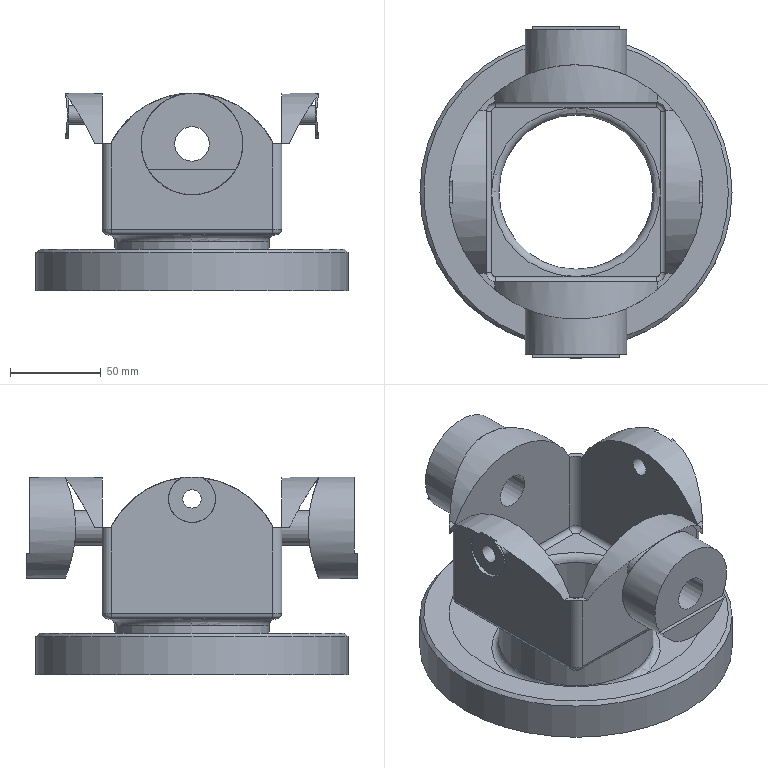Part | NX | features DATUM_CSYS 13, SKETCH 12, EXTRACT_DATUM_AXIS 10, EXTRUDE 9, EXTRACT_DATUM_PLANE 8, EXTRACT_FACE 6, HOLE PACKAGE 5, Instance Feature 5, EXTRACT_STRING 4, BLEND 3, SIMPLE HOLE 3, CBORE_HOLE 2, Intersection Curve 2, Mirror Feature 2, SYMBOLIC_THREAD 2, CHAMFER 1, DATUM_PLANE 1, Pattern Feature 1, SUBTRACT 1, SWP104 1 | 1 solid | 52 faces | box 172 x 182.995 x 109 mm | volume 961587 mm3 | cylinder 23 | plane 22 | torus 6 | cone 1 | commonest cylinder face diameters 6 x4 10 x4 100 x4 10.106 x2 19 x2 26 x2